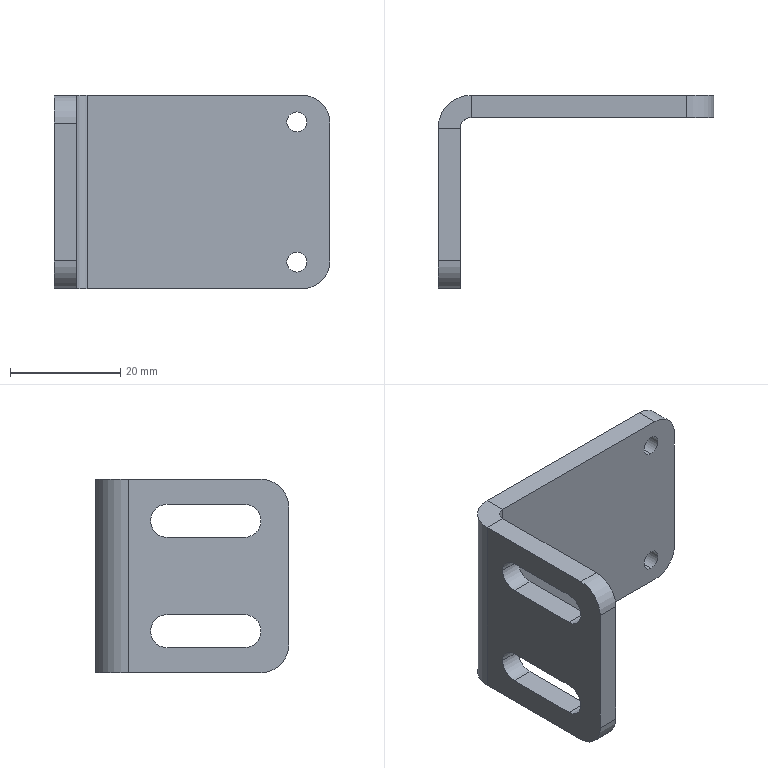Part | SolidWorks | features BaseBody 1 | 1 solid | 32 faces | box 50 x 35 x 35 mm | volume 10034 mm3 | cylinder 16 | plane 16 | commonest cylinder face diameters 6 x6 3.6 x4 10 x4 4 x1 12 x1
STEP:
#1=CARTESIAN_POINT('',(0.,-13.,10.5));
#2=VERTEX_POINT('',#1);
#3=CARTESIAN_POINT('',(0.,-10.,7.5));
#4=VERTEX_POINT('',#3);
#5=CARTESIAN_POINT('',(0.,-13.,7.5));
#6=DIRECTION('',(-1.,0.,0.));
#7=DIRECTION('',(0.,-1.,0.));
#8=AXIS2_PLACEMENT_3D('',#5,#6,#7);
#9=CIRCLE('',#8,3.);
#10=EDGE_CURVE('',#2,#4,#9,.T.);
#11=ORIENTED_EDGE('',*,*,#10,.T.);
#12=CARTESIAN_POINT('',(4.,-10.,7.5));
#13=VERTEX_POINT('',#12);
#14=CARTESIAN_POINT('',(-6.,-10.,7.5));
#15=DIRECTION('',(1.,0.,0.));
#16=VECTOR('',#15,1000.);
#17=LINE('',#14,#16);
#18=EDGE_CURVE('',#4,#13,#17,.T.);
#19=ORIENTED_EDGE('',*,*,#18,.T.);
#20=CARTESIAN_POINT('',(4.,-13.,10.5));
#21=VERTEX_POINT('',#20);
#22=CARTESIAN_POINT('',(4.,-13.,7.5));
#23=DIRECTION('',(1.,0.,0.));
#24=DIRECTION('',(0.,1.,0.));
#25=AXIS2_PLACEMENT_3D('',#22,#23,#24);
#26=CIRCLE('',#25,3.);
#27=EDGE_CURVE('',#13,#21,#26,.T.);
#28=ORIENTED_EDGE('',*,*,#27,.T.);
#29=CARTESIAN_POINT('',(-6.,-13.,10.5));
#30=DIRECTION('',(1.,0.,0.));
#31=VECTOR('',#30,1000.);
#32=LINE('',#29,#31);
#33=EDGE_CURVE('',#2,#21,#32,.T.);
#34=ORIENTED_EDGE('',*,*,#33,.F.);
#35=EDGE_LOOP('',(#11,#19,#28,#34));
#36=FACE_OUTER_BOUND('',#35,.T.);
#37=CARTESIAN_POINT('',(-6.,-13.,7.5));
#38=DIRECTION('',(1.,0.,0.));
#39=DIRECTION('',(0.,1.,0.));
#40=AXIS2_PLACEMENT_3D('',#37,#38,#39);
#41=CYLINDRICAL_SURFACE('',#40,3.);
#42=ADVANCED_FACE('',(#36),#41,.F.);
#43=CARTESIAN_POINT('',(0.,-13.,30.5));
#44=VERTEX_POINT('',#43);
#45=CARTESIAN_POINT('',(0.,-10.,27.5));
#46=VERTEX_POINT('',#45);
#47=CARTESIAN_POINT('',(0.,-13.,27.5));
#48=DIRECTION('',(-1.,0.,0.));
#49=DIRECTION('',(0.,-1.,0.));
#50=AXIS2_PLACEMENT_3D('',#47,#48,#49);
#51=CIRCLE('',#50,3.);
#52=EDGE_CURVE('',#44,#46,#51,.T.);
#53=ORIENTED_EDGE('',*,*,#52,.T.);
#54=CARTESIAN_POINT('',(4.,-10.,27.5));
#55=VERTEX_POINT('',#54);
#56=CARTESIAN_POINT('',(-6.,-10.,27.5));
#57=DIRECTION('',(1.,0.,0.));
#58=VECTOR('',#57,1000.);
#59=LINE('',#56,#58);
#60=EDGE_CURVE('',#46,#55,#59,.T.);
#61=ORIENTED_EDGE('',*,*,#60,.T.);
#62=CARTESIAN_POINT('',(4.,-13.,30.5));
#63=VERTEX_POINT('',#62);
#64=CARTESIAN_POINT('',(4.,-13.,27.5));
#65=DIRECTION('',(1.,0.,0.));
#66=DIRECTION('',(0.,-1.,0.));
#67=AXIS2_PLACEMENT_3D('',#64,#65,#66);
#68=CIRCLE('',#67,3.);
#69=EDGE_CURVE('',#55,#63,#68,.T.);
#70=ORIENTED_EDGE('',*,*,#69,.T.);
#71=CARTESIAN_POINT('',(-6.,-13.,30.5));
#72=DIRECTION('',(1.,0.,0.));
#73=VECTOR('',#72,1000.);
#74=LINE('',#71,#73);
#75=EDGE_CURVE('',#44,#63,#74,.T.);
#76=ORIENTED_EDGE('',*,*,#75,.F.);
#77=EDGE_LOOP('',(#53,#61,#70,#76));
#78=FACE_OUTER_BOUND('',#77,.T.);
#79=CARTESIAN_POINT('',(-6.,-13.,27.5));
#80=DIRECTION('',(1.,0.,0.));
#81=DIRECTION('',(0.,1.,0.));
#82=AXIS2_PLACEMENT_3D('',#79,#80,#81);
#83=CYLINDRICAL_SURFACE('',#82,3.);
#84=ADVANCED_FACE('',(#78),#83,.F.);
#85=CARTESIAN_POINT('',(44.,-4.,28.4));
#86=VERTEX_POINT('',#85);
#87=CARTESIAN_POINT('',(44.,-4.,32.));
#88=VERTEX_POINT('',#87);
#89=CARTESIAN_POINT('',(44.,-4.,30.2));
#90=DIRECTION('',(0.,1.,0.));
#91=DIRECTION('',(0.,0.,1.));
#92=AXIS2_PLACEMENT_3D('',#89,#90,#91);
#93=CIRCLE('',#92,1.8);
#94=EDGE_CURVE('',#86,#88,#93,.T.);
#95=ORIENTED_EDGE('',*,*,#94,.F.);
#96=CARTESIAN_POINT('',(44.,0.,28.4));
#97=VERTEX_POINT('',#96);
#98=CARTESIAN_POINT('',(44.,0.,28.4));
#99=DIRECTION('',(0.,1.,0.));
#100=VECTOR('',#99,1000.);
#101=LINE('',#98,#100);
#102=EDGE_CURVE('',#86,#97,#101,.T.);
#103=ORIENTED_EDGE('',*,*,#102,.T.);
#104=CARTESIAN_POINT('',(44.,0.,32.));
#105=VERTEX_POINT('',#104);
#106=CARTESIAN_POINT('',(44.,0.,30.2));
#107=DIRECTION('',(0.,1.,0.));
#108=DIRECTION('',(0.,0.,1.));
#109=AXIS2_PLACEMENT_3D('',#106,#107,#108);
#110=CIRCLE('',#109,1.8);
#111=EDGE_CURVE('',#97,#105,#110,.T.);
#112=ORIENTED_EDGE('',*,*,#111,.T.);
#113=CARTESIAN_POINT('',(44.,0.,32.));
#114=DIRECTION('',(0.,1.,0.));
#115=VECTOR('',#114,1000.);
#116=LINE('',#113,#115);
#117=EDGE_CURVE('',#88,#105,#116,.T.);
#118=ORIENTED_EDGE('',*,*,#117,.F.);
#119=EDGE_LOOP('',(#95,#103,#112,#118));
#120=FACE_OUTER_BOUND('',#119,.T.);
#121=CARTESIAN_POINT('',(44.,0.,30.2));
#122=DIRECTION('',(0.,1.,0.));
#123=DIRECTION('',(0.,0.,1.));
#124=AXIS2_PLACEMENT_3D('',#121,#122,#123);
#125=CYLINDRICAL_SURFACE('',#124,1.8);
#126=ADVANCED_FACE('',(#120),#125,.F.);
#127=CARTESIAN_POINT('',(44.,-4.,3.));
#128=VERTEX_POINT('',#127);
#129=CARTESIAN_POINT('',(44.,-4.,6.6));
#130=VERTEX_POINT('',#129);
#131=CARTESIAN_POINT('',(44.,-4.,4.8));
#132=DIRECTION('',(0.,1.,0.));
#133=DIRECTION('',(0.,0.,1.));
#134=AXIS2_PLACEMENT_3D('',#131,#132,#133);
#135=CIRCLE('',#134,1.8);
#136=EDGE_CURVE('',#128,#130,#135,.T.);
#137=ORIENTED_EDGE('',*,*,#136,.F.);
#138=CARTESIAN_POINT('',(44.,0.,3.));
#139=VERTEX_POINT('',#138);
#140=CARTESIAN_POINT('',(44.,0.,3.));
#141=DIRECTION('',(0.,1.,0.));
#142=VECTOR('',#141,1000.);
#143=LINE('',#140,#142);
#144=EDGE_CURVE('',#128,#139,#143,.T.);
#145=ORIENTED_EDGE('',*,*,#144,.T.);
#146=CARTESIAN_POINT('',(44.,0.,6.6));
#147=VERTEX_POINT('',#146);
#148=CARTESIAN_POINT('',(44.,0.,4.8));
#149=DIRECTION('',(0.,1.,0.));
#150=DIRECTION('',(0.,0.,1.));
#151=AXIS2_PLACEMENT_3D('',#148,#149,#150);
#152=CIRCLE('',#151,1.8);
#153=EDGE_CURVE('',#139,#147,#152,.T.);
#154=ORIENTED_EDGE('',*,*,#153,.T.);
#155=CARTESIAN_POINT('',(44.,0.,6.6));
#156=DIRECTION('',(0.,1.,0.));
#157=VECTOR('',#156,1000.);
#158=LINE('',#155,#157);
#159=EDGE_CURVE('',#130,#147,#158,.T.);
#160=ORIENTED_EDGE('',*,*,#159,.F.);
#161=EDGE_LOOP('',(#137,#145,#154,#160));
#162=FACE_OUTER_BOUND('',#161,.T.);
#163=CARTESIAN_POINT('',(44.,0.,4.8));
#164=DIRECTION('',(0.,1.,0.));
#165=DIRECTION('',(0.,0.,1.));
#166=AXIS2_PLACEMENT_3D('',#163,#164,#165);
#167=CYLINDRICAL_SURFACE('',#166,1.8);
#168=ADVANCED_FACE('',(#162),#167,.F.);
#169=CARTESIAN_POINT('',(44.,-4.,4.8));
#170=DIRECTION('',(0.,1.,0.));
#171=DIRECTION('',(0.,0.,1.));
#172=AXIS2_PLACEMENT_3D('',#169,#170,#171);
#173=CIRCLE('',#172,1.8);
#174=EDGE_CURVE('',#130,#128,#173,.T.);
#175=ORIENTED_EDGE('',*,*,#174,.T.);
#176=ORIENTED_EDGE('',*,*,#136,.T.);
#177=EDGE_LOOP('',(#175,#176));
#178=FACE_BOUND('',#177,.T.);
#179=CARTESIAN_POINT('',(44.,-4.,30.2));
#180=DIRECTION('',(0.,1.,0.));
#181=DIRECTION('',(0.,0.,1.));
#182=AXIS2_PLACEMENT_3D('',#179,#180,#181);
#183=CIRCLE('',#182,1.8);
#184=EDGE_CURVE('',#88,#86,#183,.T.);
#185=ORIENTED_EDGE('',*,*,#184,.T.);
#186=ORIENTED_EDGE('',*,*,#94,.T.);
#187=EDGE_LOOP('',(#185,#186));
#188=FACE_BOUND('',#187,.T.);
#189=CARTESIAN_POINT('',(6.,-4.,0.));
#190=VERTEX_POINT('',#189);
#191=CARTESIAN_POINT('',(45.,-4.,0.));
#192=VERTEX_POINT('',#191);
#193=CARTESIAN_POINT('',(0.,-4.,0.));
#194=DIRECTION('',(1.,0.,0.));
#195=VECTOR('',#194,1000.);
#196=LINE('',#193,#195);
#197=EDGE_CURVE('',#190,#192,#196,.T.);
#198=ORIENTED_EDGE('',*,*,#197,.T.);
#199=CARTESIAN_POINT('',(50.,-4.,5.));
#200=VERTEX_POINT('',#199);
#201=CARTESIAN_POINT('',(45.,-4.,5.));
#202=DIRECTION('',(0.,-1.,0.));
#203=DIRECTION('',(0.,0.,1.));
#204=AXIS2_PLACEMENT_3D('',#201,#202,#203);
#205=CIRCLE('',#204,5.);
#206=EDGE_CURVE('',#192,#200,#205,.T.);
#207=ORIENTED_EDGE('',*,*,#206,.T.);
#208=CARTESIAN_POINT('',(50.,-4.,30.));
#209=VERTEX_POINT('',#208);
#210=CARTESIAN_POINT('',(50.,-4.,35.));
#211=DIRECTION('',(0.,0.,-1.));
#212=VECTOR('',#211,1000.);
#213=LINE('',#210,#212);
#214=EDGE_CURVE('',#209,#200,#213,.T.);
#215=ORIENTED_EDGE('',*,*,#214,.F.);
#216=CARTESIAN_POINT('',(45.,-4.,35.));
#217=VERTEX_POINT('',#216);
#218=CARTESIAN_POINT('',(45.,-4.,30.));
#219=DIRECTION('',(0.,-1.,0.));
#220=DIRECTION('',(0.,0.,1.));
#221=AXIS2_PLACEMENT_3D('',#218,#219,#220);
#222=CIRCLE('',#221,5.);
#223=EDGE_CURVE('',#209,#217,#222,.T.);
#224=ORIENTED_EDGE('',*,*,#223,.T.);
#225=CARTESIAN_POINT('',(6.,-4.,35.));
#226=VERTEX_POINT('',#225);
#227=CARTESIAN_POINT('',(0.,-4.,35.));
#228=DIRECTION('',(1.,0.,0.));
#229=VECTOR('',#228,1000.);
#230=LINE('',#227,#229);
#231=EDGE_CURVE('',#226,#217,#230,.T.);
#232=ORIENTED_EDGE('',*,*,#231,.F.);
#233=CARTESIAN_POINT('',(6.,-4.,0.));
#234=DIRECTION('',(0.,0.,1.));
#235=VECTOR('',#234,1000.);
#236=LINE('',#233,#235);
#237=EDGE_CURVE('',#190,#226,#236,.T.);
#238=ORIENTED_EDGE('',*,*,#237,.F.);
#239=EDGE_LOOP('',(#198,#207,#215,#224,#232,#238));
#240=FACE_OUTER_BOUND('',#239,.T.);
#241=CARTESIAN_POINT('',(0.,-4.,35.));
#242=DIRECTION('',(0.,1.,0.));
#243=DIRECTION('',(0.,0.,1.));
#244=AXIS2_PLACEMENT_3D('',#241,#242,#243);
#245=PLANE('',#244);
#246=ADVANCED_FACE('',(#178,#188,#240),#245,.F.);
#247=CARTESIAN_POINT('',(44.,0.,30.2));
#248=DIRECTION('',(0.,1.,0.));
#249=DIRECTION('',(0.,0.,1.));
#250=AXIS2_PLACEMENT_3D('',#247,#248,#249);
#251=CIRCLE('',#250,1.8);
#252=EDGE_CURVE('',#105,#97,#251,.T.);
#253=ORIENTED_EDGE('',*,*,#252,.F.);
#254=ORIENTED_EDGE('',*,*,#111,.F.);
#255=EDGE_LOOP('',(#253,#254));
#256=FACE_BOUND('',#255,.T.);
#257=CARTESIAN_POINT('',(44.,0.,4.8));
#258=DIRECTION('',(0.,1.,0.));
#259=DIRECTION('',(0.,0.,1.));
#260=AXIS2_PLACEMENT_3D('',#257,#258,#259);
#261=CIRCLE('',#260,1.8);
#262=EDGE_CURVE('',#147,#139,#261,.T.);
#263=ORIENTED_EDGE('',*,*,#262,.F.);
#264=ORIENTED_EDGE('',*,*,#153,.F.);
#265=EDGE_LOOP('',(#263,#264));
#266=FACE_BOUND('',#265,.T.);
#267=CARTESIAN_POINT('',(50.,0.,30.));
#268=VERTEX_POINT('',#267);
#269=CARTESIAN_POINT('',(50.,0.,5.));
#270=VERTEX_POINT('',#269);
#271=CARTESIAN_POINT('',(50.,0.,35.));
#272=DIRECTION('',(0.,0.,-1.));
#273=VECTOR('',#272,1000.);
#274=LINE('',#271,#273);
#275=EDGE_CURVE('',#268,#270,#274,.T.);
#276=ORIENTED_EDGE('',*,*,#275,.T.);
#277=CARTESIAN_POINT('',(45.,0.,0.));
#278=VERTEX_POINT('',#277);
#279=CARTESIAN_POINT('',(45.,0.,5.));
#280=DIRECTION('',(0.,1.,0.));
#281=DIRECTION('',(0.,0.,1.));
#282=AXIS2_PLACEMENT_3D('',#279,#280,#281);
#283=CIRCLE('',#282,5.);
#284=EDGE_CURVE('',#270,#278,#283,.T.);
#285=ORIENTED_EDGE('',*,*,#284,.T.);
#286=CARTESIAN_POINT('',(6.,0.,0.));
#287=VERTEX_POINT('',#286);
#288=CARTESIAN_POINT('',(0.,0.,0.));
#289=DIRECTION('',(1.,0.,0.));
#290=VECTOR('',#289,1000.);
#291=LINE('',#288,#290);
#292=EDGE_CURVE('',#287,#278,#291,.T.);
#293=ORIENTED_EDGE('',*,*,#292,.F.);
#294=CARTESIAN_POINT('',(6.,0.,35.));
#295=VERTEX_POINT('',#294);
#296=CARTESIAN_POINT('',(6.,0.,0.));
#297=DIRECTION('',(0.,0.,1.));
#298=VECTOR('',#297,1000.);
#299=LINE('',#296,#298);
#300=EDGE_CURVE('',#287,#295,#299,.T.);
#301=ORIENTED_EDGE('',*,*,#300,.T.);
#302=CARTESIAN_POINT('',(45.,0.,35.));
#303=VERTEX_POINT('',#302);
#304=CARTESIAN_POINT('',(0.,0.,35.));
#305=DIRECTION('',(1.,0.,0.));
#306=VECTOR('',#305,1000.);
#307=LINE('',#304,#306);
#308=EDGE_CURVE('',#295,#303,#307,.T.);
#309=ORIENTED_EDGE('',*,*,#308,.T.);
#310=CARTESIAN_POINT('',(45.,0.,30.));
#311=DIRECTION('',(0.,1.,0.));
#312=DIRECTION('',(0.,0.,1.));
#313=AXIS2_PLACEMENT_3D('',#310,#311,#312);
#314=CIRCLE('',#313,5.);
#315=EDGE_CURVE('',#303,#268,#314,.T.);
#316=ORIENTED_EDGE('',*,*,#315,.T.);
#317=EDGE_LOOP('',(#276,#285,#293,#301,#309,#316));
#318=FACE_OUTER_BOUND('',#317,.T.);
#319=CARTESIAN_POINT('',(0.,0.,35.));
#320=DIRECTION('',(0.,1.,0.));
#321=DIRECTION('',(0.,0.,1.));
#322=AXIS2_PLACEMENT_3D('',#319,#320,#321);
#323=PLANE('',#322);
#324=ADVANCED_FACE('',(#256,#266,#318),#323,.T.);
#325=ORIENTED_EDGE('',*,*,#231,.T.);
#326=CARTESIAN_POINT('',(45.,0.,35.));
#327=DIRECTION('',(0.,1.,0.));
#328=VECTOR('',#327,1000.);
#329=LINE('',#326,#328);
#330=EDGE_CURVE('',#217,#303,#329,.T.);
#331=ORIENTED_EDGE('',*,*,#330,.T.);
#332=ORIENTED_EDGE('',*,*,#308,.F.);
#333=CARTESIAN_POINT('',(6.,-4.,35.));
#334=DIRECTION('',(0.,1.,0.));
#335=VECTOR('',#334,1000.);
#336=LINE('',#333,#335);
#337=EDGE_CURVE('',#226,#295,#336,.T.);
#338=ORIENTED_EDGE('',*,*,#337,.F.);
#339=EDGE_LOOP('',(#325,#331,#332,#338));
#340=FACE_OUTER_BOUND('',#339,.T.);
#341=CARTESIAN_POINT('',(0.,0.,35.));
#342=DIRECTION('',(0.,0.,-1.));
#343=DIRECTION('',(-1.,0.,0.));
#344=AXIS2_PLACEMENT_3D('',#341,#342,#343);
#345=PLANE('',#344);
#346=ADVANCED_FACE('',(#340),#345,.F.);
#347=ORIENTED_EDGE('',*,*,#292,.T.);
#348=CARTESIAN_POINT('',(45.,0.,0.));
#349=DIRECTION('',(0.,-1.,0.));
#350=VECTOR('',#349,1000.);
#351=LINE('',#348,#350);
#352=EDGE_CURVE('',#278,#192,#351,.T.);
#353=ORIENTED_EDGE('',*,*,#352,.T.);
#354=ORIENTED_EDGE('',*,*,#197,.F.);
#355=CARTESIAN_POINT('',(6.,-4.,0.));
#356=DIRECTION('',(0.,1.,0.));
#357=VECTOR('',#356,1000.);
#358=LINE('',#355,#357);
#359=EDGE_CURVE('',#190,#287,#358,.T.);
#360=ORIENTED_EDGE('',*,*,#359,.T.);
#361=EDGE_LOOP('',(#347,#353,#354,#360));
#362=FACE_OUTER_BOUND('',#361,.T.);
#363=CARTESIAN_POINT('',(0.,0.,0.));
#364=DIRECTION('',(0.,0.,-1.));
#365=DIRECTION('',(-1.,0.,0.));
#366=AXIS2_PLACEMENT_3D('',#363,#364,#365);
#367=PLANE('',#366);
#368=ADVANCED_FACE('',(#362),#367,.T.);
#369=ORIENTED_EDGE('',*,*,#214,.T.);
#370=CARTESIAN_POINT('',(50.,0.,5.));
#371=DIRECTION('',(0.,1.,0.));
#372=VECTOR('',#371,1000.);
#373=LINE('',#370,#372);
#374=EDGE_CURVE('',#200,#270,#373,.T.);
#375=ORIENTED_EDGE('',*,*,#374,.T.);
#376=ORIENTED_EDGE('',*,*,#275,.F.);
#377=CARTESIAN_POINT('',(50.,-4.,30.));
#378=DIRECTION('',(0.,-1.,0.));
#379=VECTOR('',#378,1000.);
#380=LINE('',#377,#379);
#381=EDGE_CURVE('',#268,#209,#380,.T.);
#382=ORIENTED_EDGE('',*,*,#381,.T.);
#383=EDGE_LOOP('',(#369,#375,#376,#382));
#384=FACE_OUTER_BOUND('',#383,.T.);
#385=CARTESIAN_POINT('',(50.,0.,35.));
#386=DIRECTION('',(1.,0.,0.));
#387=DIRECTION('',(0.,0.,-1.));
#388=AXIS2_PLACEMENT_3D('',#385,#386,#387);
#389=PLANE('',#388);
#390=ADVANCED_FACE('',(#384),#389,.T.);
#391=ORIENTED_EDGE('',*,*,#144,.F.);
#392=ORIENTED_EDGE('',*,*,#174,.F.);
#393=ORIENTED_EDGE('',*,*,#159,.T.);
#394=ORIENTED_EDGE('',*,*,#262,.T.);
#395=EDGE_LOOP('',(#391,#392,#393,#394));
#396=FACE_OUTER_BOUND('',#395,.T.);
#397=CARTESIAN_POINT('',(44.,0.,4.8));
#398=DIRECTION('',(0.,1.,0.));
#399=DIRECTION('',(0.,0.,1.));
#400=AXIS2_PLACEMENT_3D('',#397,#398,#399);
#401=CYLINDRICAL_SURFACE('',#400,1.8);
#402=ADVANCED_FACE('',(#396),#401,.F.);
#403=ORIENTED_EDGE('',*,*,#102,.F.);
#404=ORIENTED_EDGE('',*,*,#184,.F.);
#405=ORIENTED_EDGE('',*,*,#117,.T.);
#406=ORIENTED_EDGE('',*,*,#252,.T.);
#407=EDGE_LOOP('',(#403,#404,#405,#406));
#408=FACE_OUTER_BOUND('',#407,.T.);
#409=CARTESIAN_POINT('',(44.,0.,30.2));
#410=DIRECTION('',(0.,1.,0.));
#411=DIRECTION('',(0.,0.,1.));
#412=AXIS2_PLACEMENT_3D('',#409,#410,#411);
#413=CYLINDRICAL_SURFACE('',#412,1.8);
#414=ADVANCED_FACE('',(#408),#413,.F.);
#415=CARTESIAN_POINT('',(4.,-6.,35.));
#416=VERTEX_POINT('',#415);
#417=CARTESIAN_POINT('',(0.,-6.,35.));
#418=VERTEX_POINT('',#417);
#419=CARTESIAN_POINT('',(0.,-6.,35.));
#420=DIRECTION('',(-1.,0.,0.));
#421=VECTOR('',#420,1000.);
#422=LINE('',#419,#421);
#423=EDGE_CURVE('',#416,#418,#422,.T.);
#424=ORIENTED_EDGE('',*,*,#423,.F.);
#425=CARTESIAN_POINT('',(6.,-6.,35.));
#426=DIRECTION('',(0.,0.,1.));
#427=DIRECTION('',(-1.,0.,0.));
#428=AXIS2_PLACEMENT_3D('',#425,#426,#427);
#429=CIRCLE('',#428,2.);
#430=EDGE_CURVE('',#226,#416,#429,.T.);
#431=ORIENTED_EDGE('',*,*,#430,.F.);
#432=ORIENTED_EDGE('',*,*,#337,.T.);
#433=CARTESIAN_POINT('',(6.,-6.,35.));
#434=DIRECTION('',(0.,0.,1.));
#435=DIRECTION('',(-1.,0.,0.));
#436=AXIS2_PLACEMENT_3D('',#433,#434,#435);
#437=CIRCLE('',#436,6.);
#438=EDGE_CURVE('',#295,#418,#437,.T.);
#439=ORIENTED_EDGE('',*,*,#438,.T.);
#440=EDGE_LOOP('',(#424,#431,#432,#439));
#441=FACE_OUTER_BOUND('',#440,.T.);
#442=CARTESIAN_POINT('',(6.,-6.,35.));
#443=DIRECTION('',(0.,0.,1.));
#444=DIRECTION('',(1.,0.,0.));
#445=AXIS2_PLACEMENT_3D('',#442,#443,#444);
#446=PLANE('',#445);
#447=ADVANCED_FACE('',(#441),#446,.T.);
#448=CARTESIAN_POINT('',(4.,-6.,0.));
#449=VERTEX_POINT('',#448);
#450=CARTESIAN_POINT('',(6.,-6.,0.));
#451=DIRECTION('',(0.,0.,-1.));
#452=DIRECTION('',(-1.,0.,0.));
#453=AXIS2_PLACEMENT_3D('',#450,#451,#452);
#454=CIRCLE('',#453,2.);
#455=EDGE_CURVE('',#449,#190,#454,.T.);
#456=ORIENTED_EDGE('',*,*,#455,.F.);
#457=CARTESIAN_POINT('',(0.,-6.,0.));
#458=VERTEX_POINT('',#457);
#459=CARTESIAN_POINT('',(4.,-6.,0.));
#460=DIRECTION('',(-1.,0.,0.));
#461=VECTOR('',#460,1000.);
#462=LINE('',#459,#461);
#463=EDGE_CURVE('',#449,#458,#462,.T.);
#464=ORIENTED_EDGE('',*,*,#463,.T.);
#465=CARTESIAN_POINT('',(6.,-6.,0.));
#466=DIRECTION('',(0.,0.,-1.));
#467=DIRECTION('',(-1.,0.,0.));
#468=AXIS2_PLACEMENT_3D('',#465,#466,#467);
#469=CIRCLE('',#468,6.);
#470=EDGE_CURVE('',#458,#287,#469,.T.);
#471=ORIENTED_EDGE('',*,*,#470,.T.);
#472=ORIENTED_EDGE('',*,*,#359,.F.);
#473=EDGE_LOOP('',(#456,#464,#471,#472));
#474=FACE_OUTER_BOUND('',#473,.T.);
#475=CARTESIAN_POINT('',(6.,-6.,0.));
#476=DIRECTION('',(0.,0.,1.));
#477=DIRECTION('',(1.,0.,0.));
#478=AXIS2_PLACEMENT_3D('',#475,#476,#477);
#479=PLANE('',#478);
#480=ADVANCED_FACE('',(#474),#479,.F.);
#481=ORIENTED_EDGE('',*,*,#300,.F.);
#482=ORIENTED_EDGE('',*,*,#470,.F.);
#483=CARTESIAN_POINT('',(0.,-6.,0.));
#484=DIRECTION('',(0.,0.,-1.));
#485=VECTOR('',#484,1000.);
#486=LINE('',#483,#485);
#487=EDGE_CURVE('',#418,#458,#486,.T.);
#488=ORIENTED_EDGE('',*,*,#487,.F.);
#489=ORIENTED_EDGE('',*,*,#438,.F.);
#490=EDGE_LOOP('',(#481,#482,#488,#489));
#491=FACE_OUTER_BOUND('',#490,.T.);
#492=CARTESIAN_POINT('',(6.,-6.,0.));
#493=DIRECTION('',(0.,0.,-1.));
#494=DIRECTION('',(-1.,0.,0.));
#495=AXIS2_PLACEMENT_3D('',#492,#493,#494);
#496=CYLINDRICAL_SURFACE('',#495,6.);
#497=ADVANCED_FACE('',(#491),#496,.T.);
#498=ORIENTED_EDGE('',*,*,#237,.T.);
#499=ORIENTED_EDGE('',*,*,#430,.T.);
#500=CARTESIAN_POINT('',(4.,-6.,35.));
#501=DIRECTION('',(0.,0.,-1.));
#502=VECTOR('',#501,1000.);
#503=LINE('',#500,#502);
#504=EDGE_CURVE('',#416,#449,#503,.T.);
#505=ORIENTED_EDGE('',*,*,#504,.T.);
#506=ORIENTED_EDGE('',*,*,#455,.T.);
#507=EDGE_LOOP('',(#498,#499,#505,#506));
#508=FACE_OUTER_BOUND('',#507,.T.);
#509=CARTESIAN_POINT('',(6.,-6.,0.));
#510=DIRECTION('',(0.,0.,-1.));
#511=DIRECTION('',(-1.,0.,0.));
#512=AXIS2_PLACEMENT_3D('',#509,#510,#511);
#513=CYLINDRICAL_SURFACE('',#512,2.);
#514=ADVANCED_FACE('',(#508),#513,.F.);
#515=CARTESIAN_POINT('',(4.,-30.,0.));
#516=VERTEX_POINT('',#515);
#517=CARTESIAN_POINT('',(4.,0.,0.));
#518=DIRECTION('',(0.,1.,0.));
#519=VECTOR('',#518,1000.);
#520=LINE('',#517,#519);
#521=EDGE_CURVE('',#516,#449,#520,.T.);
#522=ORIENTED_EDGE('',*,*,#521,.F.);
#523=CARTESIAN_POINT('',(0.,-30.,0.));
#524=VERTEX_POINT('',#523);
#525=CARTESIAN_POINT('',(0.,-30.,0.));
#526=DIRECTION('',(-1.,0.,0.));
#527=VECTOR('',#526,1000.);
#528=LINE('',#525,#527);
#529=EDGE_CURVE('',#516,#524,#528,.T.);
#530=ORIENTED_EDGE('',*,*,#529,.T.);
#531=CARTESIAN_POINT('',(0.,-4.,0.));
#532=DIRECTION('',(0.,1.,0.));
#533=VECTOR('',#532,1000.);
#534=LINE('',#531,#533);
#535=EDGE_CURVE('',#524,#458,#534,.T.);
#536=ORIENTED_EDGE('',*,*,#535,.T.);
#537=ORIENTED_EDGE('',*,*,#463,.F.);
#538=EDGE_LOOP('',(#522,#530,#536,#537));
#539=FACE_OUTER_BOUND('',#538,.T.);
#540=CARTESIAN_POINT('',(0.,-4.,0.));
#541=DIRECTION('',(0.,0.,-1.));
#542=DIRECTION('',(-1.,0.,0.));
#543=AXIS2_PLACEMENT_3D('',#540,#541,#542);
#544=PLANE('',#543);
#545=ADVANCED_FACE('',(#539),#544,.T.);
#546=CARTESIAN_POINT('',(0.,-30.,35.));
#547=VERTEX_POINT('',#546);
#548=CARTESIAN_POINT('',(0.,-35.,35.));
#549=DIRECTION('',(0.,-1.,0.));
#550=VECTOR('',#549,1000.);
#551=LINE('',#548,#550);
#552=EDGE_CURVE('',#418,#547,#551,.T.);
#553=ORIENTED_EDGE('',*,*,#552,.T.);
#554=CARTESIAN_POINT('',(4.,-30.,35.));
#555=VERTEX_POINT('',#554);
#556=CARTESIAN_POINT('',(0.,-30.,35.));
#557=DIRECTION('',(1.,0.,0.));
#558=VECTOR('',#557,1000.);
#559=LINE('',#556,#558);
#560=EDGE_CURVE('',#547,#555,#559,.T.);
#561=ORIENTED_EDGE('',*,*,#560,.T.);
#562=CARTESIAN_POINT('',(4.,0.,35.));
#563=DIRECTION('',(0.,-1.,0.));
#564=VECTOR('',#563,1000.);
#565=LINE('',#562,#564);
#566=EDGE_CURVE('',#416,#555,#565,.T.);
#567=ORIENTED_EDGE('',*,*,#566,.F.);
#568=ORIENTED_EDGE('',*,*,#423,.T.);
#569=EDGE_LOOP('',(#553,#561,#567,#568));
#570=FACE_OUTER_BOUND('',#569,.T.);
#571=CARTESIAN_POINT('',(0.,-35.,35.));
#572=DIRECTION('',(0.,0.,1.));
#573=DIRECTION('',(1.,0.,0.));
#574=AXIS2_PLACEMENT_3D('',#571,#572,#573);
#575=PLANE('',#574);
#576=ADVANCED_FACE('',(#570),#575,.T.);
#577=ORIENTED_EDGE('',*,*,#10,.F.);
#578=CARTESIAN_POINT('',(0.,-27.,10.5));
#579=VERTEX_POINT('',#578);
#580=CARTESIAN_POINT('',(0.,0.,10.5));
#581=DIRECTION('',(0.,1.,0.));
#582=VECTOR('',#581,1000.);
#583=LINE('',#580,#582);
#584=EDGE_CURVE('',#579,#2,#583,.T.);
#585=ORIENTED_EDGE('',*,*,#584,.F.);
#586=CARTESIAN_POINT('',(0.,-27.,4.5));
#587=VERTEX_POINT('',#586);
#588=CARTESIAN_POINT('',(0.,-27.,7.5));
#589=DIRECTION('',(-1.,0.,0.));
#590=DIRECTION('',(0.,-1.,0.));
#591=AXIS2_PLACEMENT_3D('',#588,#589,#590);
#592=CIRCLE('',#591,3.);
#593=EDGE_CURVE('',#587,#579,#592,.T.);
#594=ORIENTED_EDGE('',*,*,#593,.F.);
#595=CARTESIAN_POINT('',(0.,-13.,4.5));
#596=VERTEX_POINT('',#595);
#597=CARTESIAN_POINT('',(0.,0.,4.5));
#598=DIRECTION('',(0.,-1.,0.));
#599=VECTOR('',#598,1000.);
#600=LINE('',#597,#599);
#601=EDGE_CURVE('',#596,#587,#600,.T.);
#602=ORIENTED_EDGE('',*,*,#601,.F.);
#603=CARTESIAN_POINT('',(0.,-13.,7.5));
#604=DIRECTION('',(-1.,0.,0.));
#605=DIRECTION('',(0.,-1.,0.));
#606=AXIS2_PLACEMENT_3D('',#603,#604,#605);
#607=CIRCLE('',#606,3.);
#608=EDGE_CURVE('',#4,#596,#607,.T.);
#609=ORIENTED_EDGE('',*,*,#608,.F.);
#610=EDGE_LOOP('',(#577,#585,#594,#602,#609));
#611=FACE_BOUND('',#610,.T.);
#612=ORIENTED_EDGE('',*,*,#52,.F.);
#613=CARTESIAN_POINT('',(0.,-27.,30.5));
#614=VERTEX_POINT('',#613);
#615=CARTESIAN_POINT('',(0.,0.,30.5));
#616=DIRECTION('',(0.,1.,0.));
#617=VECTOR('',#616,1000.);
#618=LINE('',#615,#617);
#619=EDGE_CURVE('',#614,#44,#618,.T.);
#620=ORIENTED_EDGE('',*,*,#619,.F.);
#621=CARTESIAN_POINT('',(0.,-27.,24.5));
#622=VERTEX_POINT('',#621);
#623=CARTESIAN_POINT('',(0.,-27.,27.5));
#624=DIRECTION('',(-1.,0.,0.));
#625=DIRECTION('',(0.,-1.,0.));
#626=AXIS2_PLACEMENT_3D('',#623,#624,#625);
#627=CIRCLE('',#626,3.);
#628=EDGE_CURVE('',#622,#614,#627,.T.);
#629=ORIENTED_EDGE('',*,*,#628,.F.);
#630=CARTESIAN_POINT('',(0.,-13.,24.5));
#631=VERTEX_POINT('',#630);
#632=CARTESIAN_POINT('',(0.,0.,24.5));
#633=DIRECTION('',(0.,-1.,0.));
#634=VECTOR('',#633,1000.);
#635=LINE('',#632,#634);
#636=EDGE_CURVE('',#631,#622,#635,.T.);
#637=ORIENTED_EDGE('',*,*,#636,.F.);
#638=CARTESIAN_POINT('',(0.,-13.,27.5));
#639=DIRECTION('',(-1.,0.,0.));
#640=DIRECTION('',(0.,-1.,0.));
#641=AXIS2_PLACEMENT_3D('',#638,#639,#640);
#642=CIRCLE('',#641,3.);
#643=EDGE_CURVE('',#46,#631,#642,.T.);
#644=ORIENTED_EDGE('',*,*,#643,.F.);
#645=EDGE_LOOP('',(#612,#620,#629,#637,#644));
#646=FACE_BOUND('',#645,.T.);
#647=CARTESIAN_POINT('',(0.,-35.,30.));
#648=VERTEX_POINT('',#647);
#649=CARTESIAN_POINT('',(0.,-35.,5.));
#650=VERTEX_POINT('',#649);
#651=CARTESIAN_POINT('',(0.,-35.,0.));
#652=DIRECTION('',(0.,0.,-1.));
#653=VECTOR('',#652,1000.);
#654=LINE('',#651,#653);
#655=EDGE_CURVE('',#648,#650,#654,.T.);
#656=ORIENTED_EDGE('',*,*,#655,.F.);
#657=CARTESIAN_POINT('',(0.,-30.,30.));
#658=DIRECTION('',(-1.,0.,0.));
#659=DIRECTION('',(0.,-1.,0.));
#660=AXIS2_PLACEMENT_3D('',#657,#658,#659);
#661=CIRCLE('',#660,5.);
#662=EDGE_CURVE('',#648,#547,#661,.T.);
#663=ORIENTED_EDGE('',*,*,#662,.T.);
#664=ORIENTED_EDGE('',*,*,#552,.F.);
#665=ORIENTED_EDGE('',*,*,#487,.T.);
#666=ORIENTED_EDGE('',*,*,#535,.F.);
#667=CARTESIAN_POINT('',(0.,-30.,5.));
#668=DIRECTION('',(-1.,0.,0.));
#669=DIRECTION('',(0.,-1.,0.));
#670=AXIS2_PLACEMENT_3D('',#667,#668,#669);
#671=CIRCLE('',#670,5.);
#672=EDGE_CURVE('',#524,#650,#671,.T.);
#673=ORIENTED_EDGE('',*,*,#672,.T.);
#674=EDGE_LOOP('',(#656,#663,#664,#665,#666,#673));
#675=FACE_OUTER_BOUND('',#674,.T.);
#676=CARTESIAN_POINT('',(0.,0.,0.));
#677=DIRECTION('',(-1.,0.,0.));
#678=DIRECTION('',(0.,-1.,0.));
#679=AXIS2_PLACEMENT_3D('',#676,#677,#678);
#680=PLANE('',#679);
#681=ADVANCED_FACE('',(#611,#646,#675),#680,.T.);
#682=CARTESIAN_POINT('',(4.,-27.,10.5));
#683=VERTEX_POINT('',#682);
#684=CARTESIAN_POINT('',(4.,-13.,10.5));
#685=DIRECTION('',(0.,-1.,0.));
#686=VECTOR('',#685,1000.);
#687=LINE('',#684,#686);
#688=EDGE_CURVE('',#21,#683,#687,.T.);
#689=ORIENTED_EDGE('',*,*,#688,.F.);
#690=ORIENTED_EDGE('',*,*,#27,.F.);
#691=CARTESIAN_POINT('',(4.,-13.,4.5));
#692=VERTEX_POINT('',#691);
#693=CARTESIAN_POINT('',(4.,-13.,7.5));
#694=DIRECTION('',(1.,0.,0.));
#695=DIRECTION('',(0.,1.,0.));
#696=AXIS2_PLACEMENT_3D('',#693,#694,#695);
#697=CIRCLE('',#696,3.);
#698=EDGE_CURVE('',#692,#13,#697,.T.);
#699=ORIENTED_EDGE('',*,*,#698,.F.);
#700=CARTESIAN_POINT('',(4.,-27.,4.5));
#701=VERTEX_POINT('',#700);
#702=CARTESIAN_POINT('',(4.,-13.,4.5));
#703=DIRECTION('',(0.,1.,0.));
#704=VECTOR('',#703,1000.);
#705=LINE('',#702,#704);
#706=EDGE_CURVE('',#701,#692,#705,.T.);
#707=ORIENTED_EDGE('',*,*,#706,.F.);
#708=CARTESIAN_POINT('',(4.,-27.,7.5));
#709=DIRECTION('',(1.,0.,0.));
#710=DIRECTION('',(0.,1.,0.));
#711=AXIS2_PLACEMENT_3D('',#708,#709,#710);
#712=CIRCLE('',#711,3.);
#713=EDGE_CURVE('',#683,#701,#712,.T.);
#714=ORIENTED_EDGE('',*,*,#713,.F.);
#715=EDGE_LOOP('',(#689,#690,#699,#707,#714));
#716=FACE_BOUND('',#715,.T.);
#717=CARTESIAN_POINT('',(4.,-27.,30.5));
#718=VERTEX_POINT('',#717);
#719=CARTESIAN_POINT('',(4.,-13.,30.5));
#720=DIRECTION('',(0.,-1.,0.));
#721=VECTOR('',#720,1000.);
#722=LINE('',#719,#721);
#723=EDGE_CURVE('',#63,#718,#722,.T.);
#724=ORIENTED_EDGE('',*,*,#723,.F.);
#725=ORIENTED_EDGE('',*,*,#69,.F.);
#726=CARTESIAN_POINT('',(4.,-13.,24.5));
#727=VERTEX_POINT('',#726);
#728=CARTESIAN_POINT('',(4.,-13.,27.5));
#729=DIRECTION('',(1.,0.,0.));
#730=DIRECTION('',(0.,-1.,0.));
#731=AXIS2_PLACEMENT_3D('',#728,#729,#730);
#732=CIRCLE('',#731,3.);
#733=EDGE_CURVE('',#727,#55,#732,.T.);
#734=ORIENTED_EDGE('',*,*,#733,.F.);
#735=CARTESIAN_POINT('',(4.,-27.,24.5));
#736=VERTEX_POINT('',#735);
#737=CARTESIAN_POINT('',(4.,-13.,24.5));
#738=DIRECTION('',(0.,1.,0.));
#739=VECTOR('',#738,1000.);
#740=LINE('',#737,#739);
#741=EDGE_CURVE('',#736,#727,#740,.T.);
#742=ORIENTED_EDGE('',*,*,#741,.F.);
#743=CARTESIAN_POINT('',(4.,-27.,27.5));
#744=DIRECTION('',(1.,0.,0.));
#745=DIRECTION('',(0.,-1.,0.));
#746=AXIS2_PLACEMENT_3D('',#743,#744,#745);
#747=CIRCLE('',#746,3.);
#748=EDGE_CURVE('',#718,#736,#747,.T.);
#749=ORIENTED_EDGE('',*,*,#748,.F.);
#750=EDGE_LOOP('',(#724,#725,#734,#742,#749));
#751=FACE_BOUND('',#750,.T.);
#752=ORIENTED_EDGE('',*,*,#566,.T.);
#753=CARTESIAN_POINT('',(4.,-35.,30.));
#754=VERTEX_POINT('',#753);
#755=CARTESIAN_POINT('',(4.,-30.,30.));
#756=DIRECTION('',(1.,0.,0.));
#757=DIRECTION('',(0.,-1.,0.));
#758=AXIS2_PLACEMENT_3D('',#755,#756,#757);
#759=CIRCLE('',#758,5.);
#760=EDGE_CURVE('',#555,#754,#759,.T.);
#761=ORIENTED_EDGE('',*,*,#760,.T.);
#762=CARTESIAN_POINT('',(4.,-35.,5.));
#763=VERTEX_POINT('',#762);
#764=CARTESIAN_POINT('',(4.,-35.,0.));
#765=DIRECTION('',(0.,0.,-1.));
#766=VECTOR('',#765,1000.);
#767=LINE('',#764,#766);
#768=EDGE_CURVE('',#754,#763,#767,.T.);
#769=ORIENTED_EDGE('',*,*,#768,.T.);
#770=CARTESIAN_POINT('',(4.,-30.,5.));
#771=DIRECTION('',(1.,0.,0.));
#772=DIRECTION('',(0.,-1.,0.));
#773=AXIS2_PLACEMENT_3D('',#770,#771,#772);
#774=CIRCLE('',#773,5.);
#775=EDGE_CURVE('',#763,#516,#774,.T.);
#776=ORIENTED_EDGE('',*,*,#775,.T.);
#777=ORIENTED_EDGE('',*,*,#521,.T.);
#778=ORIENTED_EDGE('',*,*,#504,.F.);
#779=EDGE_LOOP('',(#752,#761,#769,#776,#777,#778));
#780=FACE_OUTER_BOUND('',#779,.T.);
#781=CARTESIAN_POINT('',(4.,0.,0.));
#782=DIRECTION('',(-1.,0.,0.));
#783=DIRECTION('',(0.,-1.,0.));
#784=AXIS2_PLACEMENT_3D('',#781,#782,#783);
#785=PLANE('',#784);
#786=ADVANCED_FACE('',(#716,#751,#780),#785,.F.);
#787=ORIENTED_EDGE('',*,*,#768,.F.);
#788=CARTESIAN_POINT('',(0.,-35.,30.));
#789=DIRECTION('',(-1.,0.,0.));
#790=VECTOR('',#789,1000.);
#791=LINE('',#788,#790);
#792=EDGE_CURVE('',#754,#648,#791,.T.);
#793=ORIENTED_EDGE('',*,*,#792,.T.);
#794=ORIENTED_EDGE('',*,*,#655,.T.);
#795=CARTESIAN_POINT('',(0.,-35.,5.));
#796=DIRECTION('',(1.,0.,0.));
#797=VECTOR('',#796,1000.);
#798=LINE('',#795,#797);
#799=EDGE_CURVE('',#650,#763,#798,.T.);
#800=ORIENTED_EDGE('',*,*,#799,.T.);
#801=EDGE_LOOP('',(#787,#793,#794,#800));
#802=FACE_OUTER_BOUND('',#801,.T.);
#803=CARTESIAN_POINT('',(0.,-35.,0.));
#804=DIRECTION('',(0.,-1.,0.));
#805=DIRECTION('',(1.,0.,0.));
#806=AXIS2_PLACEMENT_3D('',#803,#804,#805);
#807=PLANE('',#806);
#808=ADVANCED_FACE('',(#802),#807,.T.);
#809=ORIENTED_EDGE('',*,*,#284,.F.);
#810=ORIENTED_EDGE('',*,*,#374,.F.);
#811=ORIENTED_EDGE('',*,*,#206,.F.);
#812=ORIENTED_EDGE('',*,*,#352,.F.);
#813=EDGE_LOOP('',(#809,#810,#811,#812));
#814=FACE_OUTER_BOUND('',#813,.T.);
#815=CARTESIAN_POINT('',(45.,0.,5.));
#816=DIRECTION('',(0.,-1.,0.));
#817=DIRECTION('',(0.,0.,-1.));
#818=AXIS2_PLACEMENT_3D('',#815,#816,#817);
#819=CYLINDRICAL_SURFACE('',#818,5.);
#820=ADVANCED_FACE('',(#814),#819,.T.);
#821=ORIENTED_EDGE('',*,*,#315,.F.);
#822=ORIENTED_EDGE('',*,*,#330,.F.);
#823=ORIENTED_EDGE('',*,*,#223,.F.);
#824=ORIENTED_EDGE('',*,*,#381,.F.);
#825=EDGE_LOOP('',(#821,#822,#823,#824));
#826=FACE_OUTER_BOUND('',#825,.T.);
#827=CARTESIAN_POINT('',(45.,0.,30.));
#828=DIRECTION('',(0.,1.,0.));
#829=DIRECTION('',(0.,0.,1.));
#830=AXIS2_PLACEMENT_3D('',#827,#828,#829);
#831=CYLINDRICAL_SURFACE('',#830,5.);
#832=ADVANCED_FACE('',(#826),#831,.T.);
#833=ORIENTED_EDGE('',*,*,#662,.F.);
#834=ORIENTED_EDGE('',*,*,#792,.F.);
#835=ORIENTED_EDGE('',*,*,#760,.F.);
#836=ORIENTED_EDGE('',*,*,#560,.F.);
#837=EDGE_LOOP('',(#833,#834,#835,#836));
#838=FACE_OUTER_BOUND('',#837,.T.);
#839=CARTESIAN_POINT('',(0.,-30.,30.));
#840=DIRECTION('',(1.,0.,0.));
#841=DIRECTION('',(0.,1.,0.));
#842=AXIS2_PLACEMENT_3D('',#839,#840,#841);
#843=CYLINDRICAL_SURFACE('',#842,5.);
#844=ADVANCED_FACE('',(#838),#843,.T.);
#845=ORIENTED_EDGE('',*,*,#672,.F.);
#846=ORIENTED_EDGE('',*,*,#529,.F.);
#847=ORIENTED_EDGE('',*,*,#775,.F.);
#848=ORIENTED_EDGE('',*,*,#799,.F.);
#849=EDGE_LOOP('',(#845,#846,#847,#848));
#850=FACE_OUTER_BOUND('',#849,.T.);
#851=CARTESIAN_POINT('',(0.,-30.,5.));
#852=DIRECTION('',(1.,0.,0.));
#853=DIRECTION('',(0.,1.,0.));
#854=AXIS2_PLACEMENT_3D('',#851,#852,#853);
#855=CYLINDRICAL_SURFACE('',#854,5.);
#856=ADVANCED_FACE('',(#850),#855,.T.);
#857=ORIENTED_EDGE('',*,*,#60,.F.);
#858=ORIENTED_EDGE('',*,*,#643,.T.);
#859=CARTESIAN_POINT('',(-6.,-13.,24.5));
#860=DIRECTION('',(1.,0.,0.));
#861=VECTOR('',#860,1000.);
#862=LINE('',#859,#861);
#863=EDGE_CURVE('',#631,#727,#862,.T.);
#864=ORIENTED_EDGE('',*,*,#863,.T.);
#865=ORIENTED_EDGE('',*,*,#733,.T.);
#866=EDGE_LOOP('',(#857,#858,#864,#865));
#867=FACE_OUTER_BOUND('',#866,.T.);
#868=CARTESIAN_POINT('',(-6.,-13.,27.5));
#869=DIRECTION('',(1.,0.,0.));
#870=DIRECTION('',(0.,1.,0.));
#871=AXIS2_PLACEMENT_3D('',#868,#869,#870);
#872=CYLINDRICAL_SURFACE('',#871,3.);
#873=ADVANCED_FACE('',(#867),#872,.F.);
#874=ORIENTED_EDGE('',*,*,#636,.T.);
#875=CARTESIAN_POINT('',(-6.,-27.,24.5));
#876=DIRECTION('',(1.,0.,0.));
#877=VECTOR('',#876,1000.);
#878=LINE('',#875,#877);
#879=EDGE_CURVE('',#622,#736,#878,.T.);
#880=ORIENTED_EDGE('',*,*,#879,.T.);
#881=ORIENTED_EDGE('',*,*,#741,.T.);
#882=ORIENTED_EDGE('',*,*,#863,.F.);
#883=EDGE_LOOP('',(#874,#880,#881,#882));
#884=FACE_OUTER_BOUND('',#883,.T.);
#885=CARTESIAN_POINT('',(-6.,-13.,24.5));
#886=DIRECTION('',(0.,0.,-1.));
#887=DIRECTION('',(0.,1.,0.));
#888=AXIS2_PLACEMENT_3D('',#885,#886,#887);
#889=PLANE('',#888);
#890=ADVANCED_FACE('',(#884),#889,.F.);
#891=ORIENTED_EDGE('',*,*,#628,.T.);
#892=CARTESIAN_POINT('',(-6.,-27.,30.5));
#893=DIRECTION('',(1.,0.,0.));
#894=VECTOR('',#893,1000.);
#895=LINE('',#892,#894);
#896=EDGE_CURVE('',#614,#718,#895,.T.);
#897=ORIENTED_EDGE('',*,*,#896,.T.);
#898=ORIENTED_EDGE('',*,*,#748,.T.);
#899=ORIENTED_EDGE('',*,*,#879,.F.);
#900=EDGE_LOOP('',(#891,#897,#898,#899));
#901=FACE_OUTER_BOUND('',#900,.T.);
#902=CARTESIAN_POINT('',(-6.,-27.,27.5));
#903=DIRECTION('',(1.,0.,0.));
#904=DIRECTION('',(0.,1.,0.));
#905=AXIS2_PLACEMENT_3D('',#902,#903,#904);
#906=CYLINDRICAL_SURFACE('',#905,3.);
#907=ADVANCED_FACE('',(#901),#906,.F.);
#908=ORIENTED_EDGE('',*,*,#619,.T.);
#909=ORIENTED_EDGE('',*,*,#75,.T.);
#910=ORIENTED_EDGE('',*,*,#723,.T.);
#911=ORIENTED_EDGE('',*,*,#896,.F.);
#912=EDGE_LOOP('',(#908,#909,#910,#911));
#913=FACE_OUTER_BOUND('',#912,.T.);
#914=CARTESIAN_POINT('',(-6.,-13.,30.5));
#915=DIRECTION('',(0.,0.,1.));
#916=DIRECTION('',(0.,-1.,0.));
#917=AXIS2_PLACEMENT_3D('',#914,#915,#916);
#918=PLANE('',#917);
#919=ADVANCED_FACE('',(#913),#918,.F.);
#920=ORIENTED_EDGE('',*,*,#18,.F.);
#921=ORIENTED_EDGE('',*,*,#608,.T.);
#922=CARTESIAN_POINT('',(-6.,-13.,4.5));
#923=DIRECTION('',(1.,0.,0.));
#924=VECTOR('',#923,1000.);
#925=LINE('',#922,#924);
#926=EDGE_CURVE('',#596,#692,#925,.T.);
#927=ORIENTED_EDGE('',*,*,#926,.T.);
#928=ORIENTED_EDGE('',*,*,#698,.T.);
#929=EDGE_LOOP('',(#920,#921,#927,#928));
#930=FACE_OUTER_BOUND('',#929,.T.);
#931=CARTESIAN_POINT('',(-6.,-13.,7.5));
#932=DIRECTION('',(1.,0.,0.));
#933=DIRECTION('',(0.,1.,0.));
#934=AXIS2_PLACEMENT_3D('',#931,#932,#933);
#935=CYLINDRICAL_SURFACE('',#934,3.);
#936=ADVANCED_FACE('',(#930),#935,.F.);
#937=ORIENTED_EDGE('',*,*,#601,.T.);
#938=CARTESIAN_POINT('',(-6.,-27.,4.5));
#939=DIRECTION('',(1.,0.,0.));
#940=VECTOR('',#939,1000.);
#941=LINE('',#938,#940);
#942=EDGE_CURVE('',#587,#701,#941,.T.);
#943=ORIENTED_EDGE('',*,*,#942,.T.);
#944=ORIENTED_EDGE('',*,*,#706,.T.);
#945=ORIENTED_EDGE('',*,*,#926,.F.);
#946=EDGE_LOOP('',(#937,#943,#944,#945));
#947=FACE_OUTER_BOUND('',#946,.T.);
#948=CARTESIAN_POINT('',(-6.,-13.,4.5));
#949=DIRECTION('',(0.,0.,-1.));
#950=DIRECTION('',(0.,1.,0.));
#951=AXIS2_PLACEMENT_3D('',#948,#949,#950);
#952=PLANE('',#951);
#953=ADVANCED_FACE('',(#947),#952,.F.);
#954=ORIENTED_EDGE('',*,*,#593,.T.);
#955=CARTESIAN_POINT('',(-6.,-27.,10.5));
#956=DIRECTION('',(1.,0.,0.));
#957=VECTOR('',#956,1000.);
#958=LINE('',#955,#957);
#959=EDGE_CURVE('',#579,#683,#958,.T.);
#960=ORIENTED_EDGE('',*,*,#959,.T.);
#961=ORIENTED_EDGE('',*,*,#713,.T.);
#962=ORIENTED_EDGE('',*,*,#942,.F.);
#963=EDGE_LOOP('',(#954,#960,#961,#962));
#964=FACE_OUTER_BOUND('',#963,.T.);
#965=CARTESIAN_POINT('',(-6.,-27.,7.5));
#966=DIRECTION('',(1.,0.,0.));
#967=DIRECTION('',(0.,1.,0.));
#968=AXIS2_PLACEMENT_3D('',#965,#966,#967);
#969=CYLINDRICAL_SURFACE('',#968,3.);
#970=ADVANCED_FACE('',(#964),#969,.F.);
#971=ORIENTED_EDGE('',*,*,#584,.T.);
#972=ORIENTED_EDGE('',*,*,#33,.T.);
#973=ORIENTED_EDGE('',*,*,#688,.T.);
#974=ORIENTED_EDGE('',*,*,#959,.F.);
#975=EDGE_LOOP('',(#971,#972,#973,#974));
#976=FACE_OUTER_BOUND('',#975,.T.);
#977=CARTESIAN_POINT('',(-6.,-13.,10.5));
#978=DIRECTION('',(0.,0.,1.));
#979=DIRECTION('',(0.,-1.,0.));
#980=AXIS2_PLACEMENT_3D('',#977,#978,#979);
#981=PLANE('',#980);
#982=ADVANCED_FACE('',(#976),#981,.F.);
#983=CLOSED_SHELL('',(#42,#84,#126,#168,#246,#324,#346,#368,#390,#402,#414,#447,#480,#497,#514,#545,#576,#681,#786,#808,#820,#832,#844,#856,#873,#890,#907,#919,#936,#953,#970,#982));
#984=MANIFOLD_SOLID_BREP('',#983);
#985=CARTESIAN_POINT('',(0.,0.,0.));
#986=DIRECTION('',(0.,0.,1.));
#987=DIRECTION('',(1.,0.,0.));
#988=AXIS2_PLACEMENT_3D('',#985,#986,#987);
#989=(LENGTH_UNIT()NAMED_UNIT(*)SI_UNIT(.MILLI.,.METRE.));
#990=UNCERTAINTY_MEASURE_WITH_UNIT(LENGTH_MEASURE(0.00001),#989,'','');
#991=(NAMED_UNIT(*)PLANE_ANGLE_UNIT()SI_UNIT($,.RADIAN.));
#992=(NAMED_UNIT(*)SI_UNIT($,.STERADIAN.)SOLID_ANGLE_UNIT());
#993=(GEOMETRIC_REPRESENTATION_CONTEXT(3)GLOBAL_UNCERTAINTY_ASSIGNED_CONTEXT((#990))GLOBAL_UNIT_ASSIGNED_CONTEXT((#989,#991,#992))REPRESENTATION_CONTEXT('',''));
#994=ADVANCED_BREP_SHAPE_REPRESENTATION('',(#984,#988),#993);